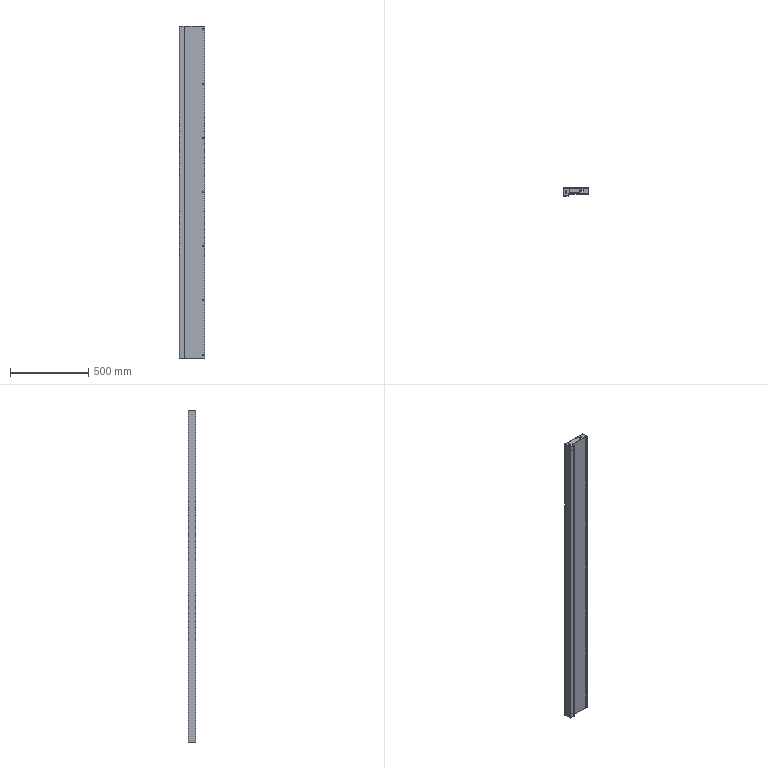Part | SolidWorks | 5 solids | 343 faces | box 160.7 x 50 x 2116 mm | volume 1348721 mm3 | plane 196 | cylinder 147 | commonest cylinder face diameters 5 x35 6.2 x28 4.2 x14 10 x14 8 x12 11 x12